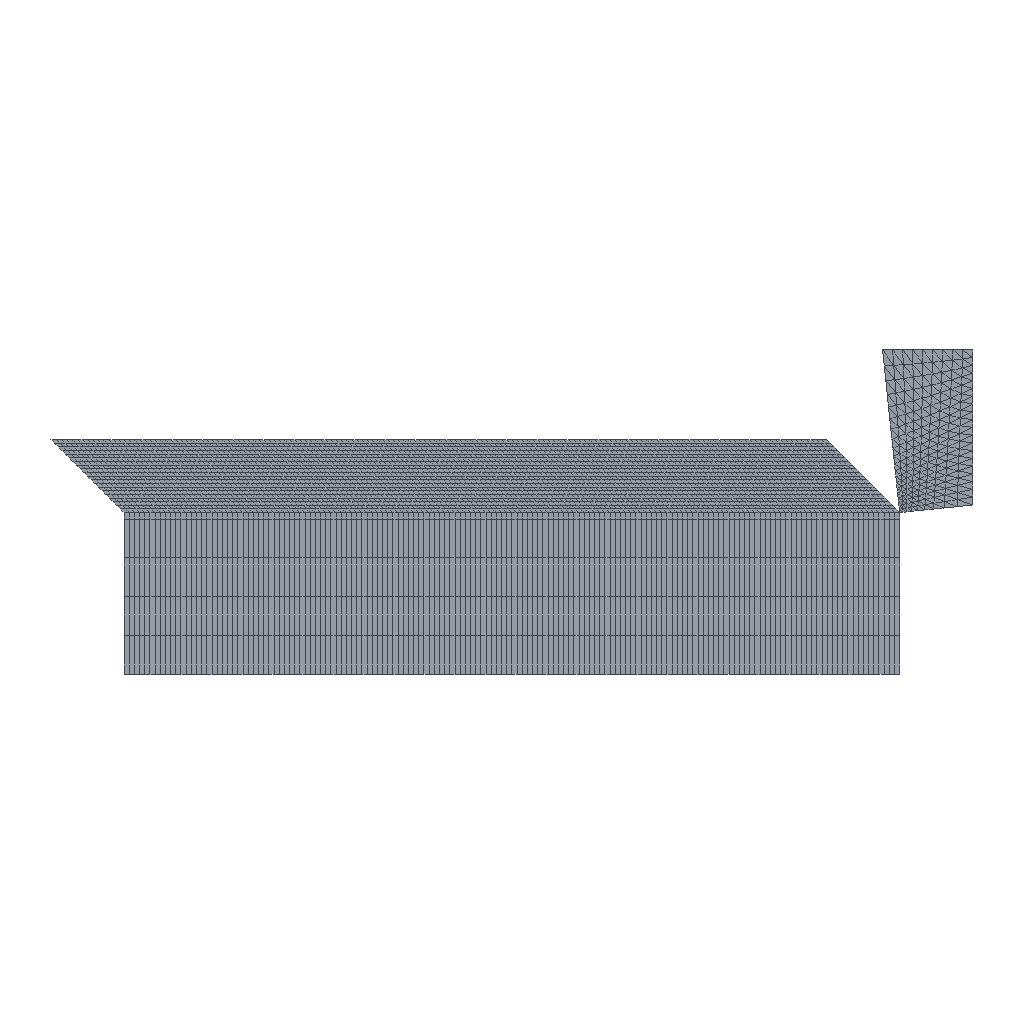Simulation study | abaqus
Set-up summary:
category,name,step,type,value,unit,region
solver,abaqus
solver,version,,,Abaqus/Explicit 2020
units,not stated in the deck,,not stated
analysis,deck,,dynamic temperature-displacement,dynamic temperature-displacement
load_step,Step-1,Step-1,dynamic temperature-displacement
load_step,requested,,,1
mesh,nodes,,,4136
mesh,elements,,,4110
element_type,CPE3T,,plane,360
element_type,CPE4RT,,plane,3750
load,load commands in deck,,count,1
bc,support commands in deck,,count,4
material,TI,,in results
material,TI-COPY,,in results
material,TI6AL4V-GAI,,in results
material,TI6AL4V-SUN,,in results
material,YG6,,in results
check,setup vs results,,match,"per instance, exact: element labels, types and connectivity; labels of the nodes the elements use; coordinates of those nodes at SINGLE_PRECISION in 2 of 2 instance(s)"
Abaqus input file, long lists of numbers shortened:
*Heading
** Job name: Job-1 Model name: Model-1
** Generated by: Abaqus/CAE 2020
*Preprint, echo=NO, model=NO, history=NO, contact=NO
**
** PARTS
**
*Part, name=Part-tool
*Node
      1, 0.05,  0.3
      2, 0.05659,  0.2373
** (208 more lines like these left out)
*Element, type=CPE3T
  1,   1,   2,  23
  2,  23,  22,   1
** (358 more lines like these left out)
*Nset, nset=Set-6, generate
   1,  210,    1
*Elset, elset=Set-6, generate
   1,  360,    1
** Section: Section-tool
*Solid Section, elset=Set-6, material=YG6
2.5,
*End Part
**
*Part, name=work
*Node
      1,          1.5, -0.2125
      2,         -1.5, -0.2125
** (3924 more lines like these left out)
*Element, type=CPE4RT
  1,    1,    9,  649,  312
  2,    9,   10,  650,  649
** (3748 more lines like these left out)
*Nset, nset=Set-4, generate
    1,  3926,     1
*Elset, elset=Set-4, generate
    1,  3750,     1
*Nset, nset=Set-12, generate
    1,  3926,     1
*Elset, elset=Set-12
    1,    2,    3,    4,    5,    6,    7,    8,    9,   10,   11,   12,   13,   14,   15,   16
   17,   18,   19,   20,   21,   22,   23,   24,   25,   26,   27,   28,   29,   30,   31,   32
** (223 more lines like these left out)
*Nset, nset=Set-13
   1,   2,   5,   6,   9,  10,  11,  12,  13,  14,  15,  16,  17,  18,  19,  20
  21,  22,  23,  24,  25,  26,  27,  28,  29,  30,  31,  32,  33,  34,  35,  36
** (17 more lines like these left out)
*Elset, elset=Set-13, generate
 601,  750,    1
** Section: ti
*Solid Section, elset=Set-12, material=ti
,
** Section: middle
*Solid Section, elset=Set-13, material=ti-Copy
,
*End Part
**
**
** ASSEMBLY
**
*Assembly, name=Assembly
**
*Instance, name=Part-tool-1, part=Part-tool
    1.384,     0.1423,           0.
*End Instance
**
*Instance, name=work-1, part=work
*End Instance
**
*Node
      1,   1.784,   0.4423,           0.
*Nset, nset=Set-9, instance=work-1, generate
    1,  3926,     1
*Elset, elset=Set-9, instance=work-1, generate
    1,  3750,     1
*Nset, nset=Set-10, instance=Part-tool-1, generate
   1,  210,    1
*Elset, elset=Set-10, instance=Part-tool-1, generate
   1,  360,    1
*Nset, nset=Set-11, instance=work-1
   2,   3,   4, 158, 159, 160, 161, 162, 163, 164, 165, 166, 167, 168, 169, 170
 171, 172, 173, 174, 175, 176, 177, 178, 179, 180, 181, 182, 183, 184, 185, 186
** (8 more lines like these left out)
*Elset, elset=Set-11, instance=work-1
 150, 300, 450, 451, 452, 453, 454, 455, 456, 457, 458, 459, 460, 461, 462, 463
 464, 465, 466, 467, 468, 469, 470, 471, 472, 473, 474, 475, 476, 477, 478, 479
** (8 more lines like these left out)
*Nset, nset=Set-RP
 1,
*Nset, nset=b_Set-7, instance=Part-tool-1, generate
   1,  210,    1
*Elset, elset=b_Set-7, instance=Part-tool-1, generate
   1,  360,    1
*Nset, nset=s_Set-12, instance=work-1
    1,    2,    5,    6,    7,    8,    9,   10,   11,   12,   13,   14,   15,   16,   17,   18
   19,   20,   21,   22,   23,   24,   25,   26,   27,   28,   29,   30,   31,   32,   33,   34
** (206 more lines like these left out)
*Elset, elset=s_Set-12, instance=work-1, generate
  601,  3750,     1
*Nset, nset=s_Set-13, instance=work-1
    1,    2,    5,    6,    7,    8,    9,   10,   11,   12,   13,   14,   15,   16,   17,   18
   19,   20,   21,   22,   23,   24,   25,   26,   27,   28,   29,   30,   31,   32,   33,   34
** (206 more lines like these left out)
*Elset, elset=s_Set-13, instance=work-1, generate
  601,  3750,     1
*Nset, nset=_PickedSet38, internal
 1,
*Elset, elset=_Surf-8_S2, internal, instance=work-1, generate
  750,  3750,   150
*Elset, elset=_Surf-8_S1, internal, instance=work-1, generate
 751,  900,    1
*Elset, elset=_Surf-8_S4, internal, instance=work-1, generate
  751,  3601,   150
*Surface, type=ELEMENT, name=Surf-8
_Surf-8_S2, S2
_Surf-8_S1, S1
_Surf-8_S4, S4
*Elset, elset=_m_Surf-7_S1, internal, instance=Part-tool-1, generate
  1,  39,   2
*Elset, elset=_m_Surf-7_S2, internal, instance=Part-tool-1
   2,  39,  42,  79,  82, 119, 122, 159, 162, 199, 202, 239, 242, 279, 282, 319
 322, 359
*Surface, type=ELEMENT, name=m_Surf-7
_m_Surf-7_S1, S1
_m_Surf-7_S2, S2
*Surface, type=NODE, name=s_Set-13_CNS_, internal
s_Set-13, 1.
** Constraint: Constraint-1
*Rigid Body, ref node=_PickedSet38, elset=b_Set-7, position=CENTER OF MASS
*End Assembly
**
** MATERIALS
**
*Material, name=TI6AL4V-gai
*Conductivity
  5.44, 20.
   6.7,100.
  8.79,200.
 10.47,300.
 12.56,400.
 14.24,500.
 15.49,600.
*Damage Initiation, criterion=JOHNSON COOK
 -0.09,  0.25, -0.48, 0.014,  3.87, 1630.,   25.,    1.
*Damage Evolution, type=DISPLACEMENT
 0.1,
*Density
 4.44e-09,
*Elastic
105000., 0.31
*Expansion
 9.4e-06,100.
 9.5e-06,200.
 9.6e-06,300.
 9.7e-06,400.
 9.9e-06,500.
   1e-05,600.
*Inelastic Heat Fraction
         0.9,
*Plastic, hardening=JOHNSON COOK
875.,  793., 0.386,  0.71, 1630.,   25.
*Rate Dependent, type=JOHNSON COOK
 0.01,1.
*Specific Heat
 5.65e+08, 20.
 6.78e+08,100.
 6.91e+08,200.
 7.03e+08,300.
 7.41e+08,400.
 7.54e+08,500.
 8.79e+08,600.
*Material, name=TI6AL4V-sun
*Conductivity
  5.44, 20.
   6.7,100.
  8.79,200.
 10.47,300.
 12.56,400.
 14.24,500.
 15.49,600.
*Damage Initiation, criterion=JOHNSON COOK
 -0.09,  0.25, -0.48, 0.014,  3.87, 1630.,   25.,    1.
*Damage Evolution, type=DISPLACEMENT
 0.15,
*Density
 4.44e-09,
*Elastic
105000., 0.31
*Expansion
 9.4e-06,100.
 9.5e-06,200.
 9.6e-06,300.
 9.7e-06,400.
 9.9e-06,500.
   1e-05,600.
*Inelastic Heat Fraction
         0.9,
*Plastic, hardening=JOHNSON COOK
875.,  793., 0.386,  0.71, 1630.,   25.
*Rate Dependent, type=JOHNSON COOK
 0.01,1.
*Specific Heat
 5.65e+08, 20.
 6.78e+08,100.
 6.91e+08,200.
 7.03e+08,300.
 7.41e+08,400.
 7.54e+08,500.
 8.79e+08,600.
*Material, name=YG6
*Conductivity
 79.6,
*Density
 1.485e-08,
*Elastic
640000., 0.22
*Expansion
 4.7e-06,
*Inelastic Heat Fraction
         0.9,
*Specific Heat
 1.76e+08,
*Material, name=ti
*Conductivity
  7.5, 20.
  8.7,200.
 11.8,500.
*Damage Initiation, criterion=JOHNSON COOK
 -0.09,  0.25,  -0.5, 0.014,  3.87, 1650.,   25.,    1.
*Damage Evolution, type=DISPLACEMENT
 0.085,
*Density
 4.44e-09,
*Elastic
108000., 0.33
*Expansion
 9.1e-06, 20.
 9.2e-06,250.
 9.7e-06,500.
*Inelastic Heat Fraction
         0.9,
*Plastic, hardening=JOHNSON COOK
860., 683., 0.47,   1.,1650.,  25.
*Rate Dependent, type=JOHNSON COOK
 0.035,1.
*Specific Heat
 5.263e+08,
*Material, name=ti-Copy
*Conductivity
  7.5, 20.
  8.7,200.
 11.8,500.
*Damage Initiation, criterion=JOHNSON COOK
 -0.09,  0.25,  -0.5, 0.014,  3.87, 1650.,   25.,    1.
*Damage Evolution, type=DISPLACEMENT
 0.04,
*Density
 4.44e-09,
*Elastic
108000., 0.33
*Expansion
 9.1e-06, 20.
 9.2e-06,250.
 9.7e-06,500.
*Inelastic Heat Fraction
         0.9,
*Plastic, hardening=JOHNSON COOK
860., 683., 0.47,   1.,1650.,  25.
*Rate Dependent, type=JOHNSON COOK
 0.035,1.
*Specific Heat
 5.263e+08,
**
** INTERACTION PROPERTIES
**
*Surface Interaction, name=IntProp-1
*Friction
 0.1,
*Surface Behavior, pressure-overclosure=HARD
*Surface Interaction, name=zijie
*Friction
 0.5,
*Surface Behavior, pressure-overclosure=HARD
**
** BOUNDARY CONDITIONS
**
** Name: BC-1 Type: 对称/反对称/完全固定
*Boundary
Set-11, ENCASTRE
**
** PREDEFINED FIELDS
**
** Name: Predefined Field-1   Type: Temperature
*Initial Conditions, type=TEMPERATURE
Set-9, 20.
** Name: Predefined Field-2   Type: Temperature
*Initial Conditions, type=TEMPERATURE
Set-10, 20.
** ----------------------------------------------------------------
**
** STEP: Step-1
**
*Step, name=Step-1, nlgeom=YES
*Dynamic Temperature-displacement, Explicit
, 0.001
*Bulk Viscosity
0.06, 1.2
** Mass Scaling: Semi-Automatic
**               Whole Model
*Fixed Mass Scaling, factor=200.
**
** BOUNDARY CONDITIONS
**
** Name: BC-2 Type: 速度/角速度
*Boundary, type=VELOCITY
Set-RP, 1, 1, -1666.
Set-RP, 2, 2
Set-RP, 6, 6
*Adaptive Mesh Controls, name=Ada-1, curvature refinement=5.
0.5, 0., 0.5
**
** INTERACTIONS
**
** Interaction: Int-1
*Contact Pair, interaction=IntProp-1, mechanical constraint=KINEMATIC, cpset=Int-1
m_Surf-7, s_Set-13_CNS_
** Interaction: Int-2
*Contact, op=NEW
*Contact Inclusions, ALL EXTERIOR
*Contact Property Assignment
 ,  , zijie
**
** OUTPUT REQUESTS
**
*Restart, write, number interval=1, time marks=NO
**
** FIELD OUTPUT: F-Output-1
**
*Output, field, number interval=100
*Node Output
A, NT, RF, RFL, U, V
*Element Output, directions=YES
E, EVF, HFL, LE, MISES, PE, PEEQ, PEEQVAVG, PEVAVG, S, STATUS, SVAVG, TEMP
*Contact Output
CSTRESS,
**
** HISTORY OUTPUT: H-Output-1
**
*Output, history, time interval=5e-07
*Node Output, nset=Set-RP
RF1, RF2, RF3
*End Step
Results summary:
result,step,Step-1,partial,increments=59281 time=0.0005892/0.001
result,analysis,,,"dynamic temperature-displacement, explict"
result,last_loadstep,,,1
result,primary field,,,"U, NT11"
result,reaction total,,FX,177.08,model units
result,reaction total,,FY,-40.811,model units
result,reaction total,,FZ,0.0,model units